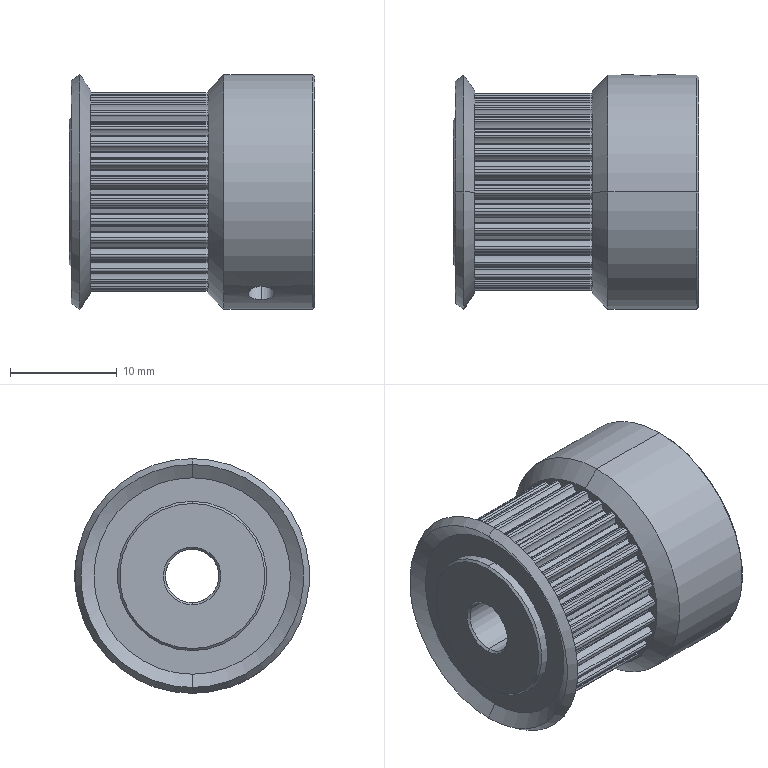Part | SolidWorks | features BaseBody 1 | 1 solid | 296 faces | box 23 x 22 x 22 mm | volume 6448 mm3 | cylinder 275 | cone 16 | plane 5 | commonest cylinder face diameters 0.38 x72 0.2 x68 2.65 x64 18.59 x31 17.07 x30 2.459 x4